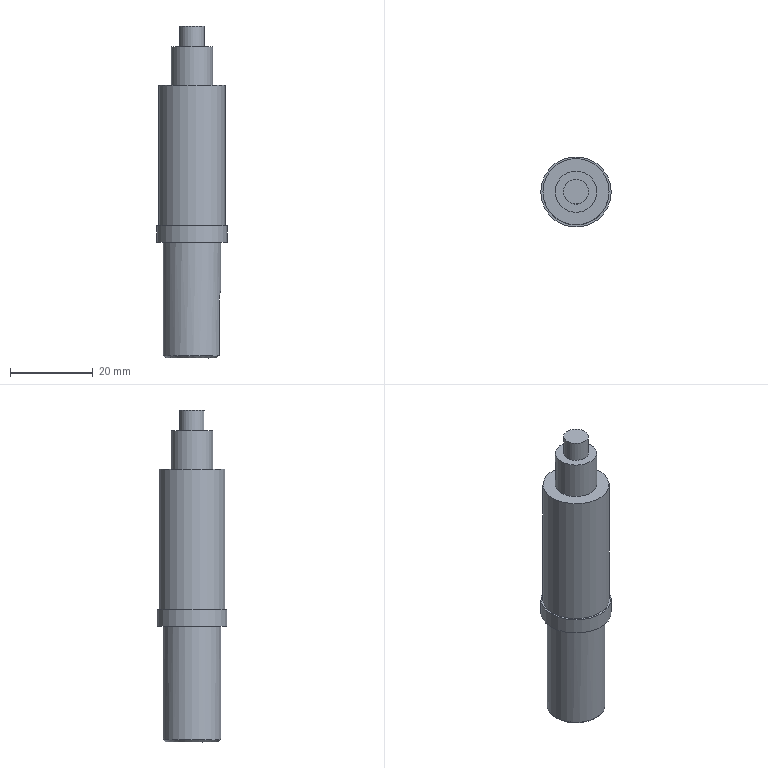Part | STEP file | 1 solid | 16 faces | box 17 x 17 x 80.2 mm | volume 12671 mm3 | plane 9 | cylinder 6 | cone 1 | commonest cylinder face diameters 5 x1 6 x1 10 x1 14 x1 16 x1 17 x1
STEP:
#1=CARTESIAN_POINT('',(0.,0.,0.));
#2=DIRECTION('',(0.,0.,1.));
#3=DIRECTION('',(1.,0.,0.));
#4=AXIS2_PLACEMENT_3D('',#1,#2,#3);
#5=CARTESIAN_POINT('',(8.,0.,-14.3));
#6=VERTEX_POINT('',#5);
#7=CARTESIAN_POINT('',(0.,0.,-14.3));
#8=DIRECTION('',(0.,0.,-1.));
#9=DIRECTION('',(1.,0.,0.));
#10=AXIS2_PLACEMENT_3D('',#7,#8,#9);
#11=CIRCLE('',#10,8.);
#12=CARTESIAN_POINT('',(0.,0.,-14.3));
#13=DIRECTION('',(0.,0.,1.));
#14=DIRECTION('',(1.,0.,0.));
#15=AXIS2_PLACEMENT_3D('',#12,#13,#14);
#16=CYLINDRICAL_SURFACE('',#15,8.);
#17=CARTESIAN_POINT('',(6.283,0.));
#18=DIRECTION('',(-1.,0.));
#19=VECTOR('',#18,1.);
#20=LINE('',#17,#19);
#21=(GEOMETRIC_REPRESENTATION_CONTEXT(2)PARAMETRIC_REPRESENTATION_CONTEXT()REPRESENTATION_CONTEXT('',''));
#22=DEFINITIONAL_REPRESENTATION('',(#20),#21);
#23=PCURVE('',#16,#22);
#24=CARTESIAN_POINT('',(0.,0.,-14.3));
#25=DIRECTION('',(0.,0.,1.));
#26=DIRECTION('',(1.,0.,0.));
#27=AXIS2_PLACEMENT_3D('',#24,#25,#26);
#28=PLANE('',#27);
#29=CARTESIAN_POINT('',(8.,0.));
#30=CARTESIAN_POINT('',(8.,-13.856));
#31=CARTESIAN_POINT('',(-4.,-6.928));
#32=CARTESIAN_POINT('',(-16.,0.));
#33=CARTESIAN_POINT('',(-4.,6.928));
#34=CARTESIAN_POINT('',(8.,13.856));
#35=CARTESIAN_POINT('',(8.,0.));
#36=(BOUNDED_CURVE()B_SPLINE_CURVE(2,(#29,#30,#31,#32,#33,#34,#35),.UNSPECIFIED.,.T.,.F.)B_SPLINE_CURVE_WITH_KNOTS((1,2,2,2,2,1),(-2.094,0.,2.094,4.189,6.283,8.378),.UNSPECIFIED.)CURVE()GEOMETRIC_REPRESENTATION_ITEM()RATIONAL_B_SPLINE_CURVE((1.,0.5,1.,0.5,1.,0.5,1.))REPRESENTATION_ITEM(''));
#37=(GEOMETRIC_REPRESENTATION_CONTEXT(2)PARAMETRIC_REPRESENTATION_CONTEXT()REPRESENTATION_CONTEXT('',''));
#38=DEFINITIONAL_REPRESENTATION('',(#36),#37);
#39=PCURVE('',#28,#38);
#40=SURFACE_CURVE('',#11,(#23,#39),.PCURVE_S1.);
#41=EDGE_CURVE('',#6,#6,#40,.T.);
#42=ORIENTED_EDGE('',*,*,#41,.T.);
#43=CARTESIAN_POINT('',(8.,0.,-48.3));
#44=VERTEX_POINT('',#43);
#45=CARTESIAN_POINT('',(8.,0.,-48.3));
#46=CARTESIAN_POINT('',(8.,0.,-14.3));
#47=B_SPLINE_CURVE_WITH_KNOTS('',1,(#45,#46),.UNSPECIFIED.,.F.,.F.,(2,2),(-34.,0.),.PIECEWISE_BEZIER_KNOTS.);
#48=CARTESIAN_POINT('',(0.,0.));
#49=DIRECTION('',(0.,1.));
#50=VECTOR('',#49,1.);
#51=LINE('',#48,#50);
#52=(GEOMETRIC_REPRESENTATION_CONTEXT(2)PARAMETRIC_REPRESENTATION_CONTEXT()REPRESENTATION_CONTEXT('',''));
#53=DEFINITIONAL_REPRESENTATION('',(#51),#52);
#54=PCURVE('',#16,#53);
#55=CARTESIAN_POINT('',(6.283,0.));
#56=DIRECTION('',(0.,1.));
#57=VECTOR('',#56,1.);
#58=LINE('',#55,#57);
#59=(GEOMETRIC_REPRESENTATION_CONTEXT(2)PARAMETRIC_REPRESENTATION_CONTEXT()REPRESENTATION_CONTEXT('',''));
#60=DEFINITIONAL_REPRESENTATION('',(#58),#59);
#61=PCURVE('',#16,#60);
#62=SEAM_CURVE('',#47,(#54,#61),.PCURVE_S1.);
#63=EDGE_CURVE('',#44,#6,#62,.T.);
#64=ORIENTED_EDGE('',*,*,#63,.F.);
#65=CARTESIAN_POINT('',(0.,0.,-48.3));
#66=DIRECTION('',(0.,0.,1.));
#67=DIRECTION('',(1.,0.,0.));
#68=AXIS2_PLACEMENT_3D('',#65,#66,#67);
#69=CIRCLE('',#68,8.);
#70=CARTESIAN_POINT('',(0.,-34.));
#71=DIRECTION('',(1.,0.));
#72=VECTOR('',#71,1.);
#73=LINE('',#70,#72);
#74=(GEOMETRIC_REPRESENTATION_CONTEXT(2)PARAMETRIC_REPRESENTATION_CONTEXT()REPRESENTATION_CONTEXT('',''));
#75=DEFINITIONAL_REPRESENTATION('',(#73),#74);
#76=PCURVE('',#16,#75);
#77=CARTESIAN_POINT('',(0.,0.,-48.3));
#78=DIRECTION('',(0.,0.,1.));
#79=DIRECTION('',(1.,0.,0.));
#80=AXIS2_PLACEMENT_3D('',#77,#78,#79);
#81=PLANE('',#80);
#82=CARTESIAN_POINT('',(0.,0.));
#83=DIRECTION('',(1.,0.));
#84=AXIS2_PLACEMENT_2D('',#82,#83);
#85=CIRCLE('',#84,8.);
#86=(GEOMETRIC_REPRESENTATION_CONTEXT(2)PARAMETRIC_REPRESENTATION_CONTEXT()REPRESENTATION_CONTEXT('',''));
#87=DEFINITIONAL_REPRESENTATION('',(#85),#86);
#88=PCURVE('',#81,#87);
#89=SURFACE_CURVE('',#69,(#76,#88),.PCURVE_S1.);
#90=EDGE_CURVE('',#44,#44,#89,.T.);
#91=ORIENTED_EDGE('',*,*,#90,.T.);
#92=ORIENTED_EDGE('',*,*,#63,.T.);
#93=EDGE_LOOP('',(#42,#64,#91,#92));
#94=FACE_BOUND('',#93,.T.);
#95=ADVANCED_FACE('',(#94),#16,.T.);
#96=CARTESIAN_POINT('',(5.,0.,-14.3));
#97=VERTEX_POINT('',#96);
#98=CARTESIAN_POINT('',(0.,0.,-14.3));
#99=DIRECTION('',(0.,0.,-1.));
#100=DIRECTION('',(1.,0.,0.));
#101=AXIS2_PLACEMENT_3D('',#98,#99,#100);
#102=CIRCLE('',#101,5.);
#103=CARTESIAN_POINT('',(5.,0.));
#104=CARTESIAN_POINT('',(5.,-8.66));
#105=CARTESIAN_POINT('',(-2.5,-4.33));
#106=CARTESIAN_POINT('',(-10.,0.));
#107=CARTESIAN_POINT('',(-2.5,4.33));
#108=CARTESIAN_POINT('',(5.,8.66));
#109=CARTESIAN_POINT('',(5.,0.));
#110=(BOUNDED_CURVE()B_SPLINE_CURVE(2,(#103,#104,#105,#106,#107,#108,#109),.UNSPECIFIED.,.T.,.F.)B_SPLINE_CURVE_WITH_KNOTS((1,2,2,2,2,1),(-2.094,0.,2.094,4.189,6.283,8.378),.UNSPECIFIED.)CURVE()GEOMETRIC_REPRESENTATION_ITEM()RATIONAL_B_SPLINE_CURVE((1.,0.5,1.,0.5,1.,0.5,1.))REPRESENTATION_ITEM(''));
#111=(GEOMETRIC_REPRESENTATION_CONTEXT(2)PARAMETRIC_REPRESENTATION_CONTEXT()REPRESENTATION_CONTEXT('',''));
#112=DEFINITIONAL_REPRESENTATION('',(#110),#111);
#113=PCURVE('',#28,#112);
#114=CARTESIAN_POINT('',(0.,0.,-5.));
#115=DIRECTION('',(0.,0.,1.));
#116=DIRECTION('',(1.,0.,0.));
#117=AXIS2_PLACEMENT_3D('',#114,#115,#116);
#118=CYLINDRICAL_SURFACE('',#117,5.);
#119=CARTESIAN_POINT('',(6.283,-9.3));
#120=DIRECTION('',(-1.,0.));
#121=VECTOR('',#120,1.);
#122=LINE('',#119,#121);
#123=(GEOMETRIC_REPRESENTATION_CONTEXT(2)PARAMETRIC_REPRESENTATION_CONTEXT()REPRESENTATION_CONTEXT('',''));
#124=DEFINITIONAL_REPRESENTATION('',(#122),#123);
#125=PCURVE('',#118,#124);
#126=SURFACE_CURVE('',#102,(#113,#125),.PCURVE_S1.);
#127=EDGE_CURVE('',#97,#97,#126,.T.);
#128=ORIENTED_EDGE('',*,*,#127,.T.);
#129=EDGE_LOOP('',(#128));
#130=FACE_BOUND('',#129,.T.);
#131=ORIENTED_EDGE('',*,*,#41,.F.);
#132=EDGE_LOOP('',(#131));
#133=FACE_BOUND('',#132,.T.);
#134=ADVANCED_FACE('',(#130,#133),#28,.T.);
#135=ORIENTED_EDGE('',*,*,#90,.F.);
#136=EDGE_LOOP('',(#135));
#137=FACE_BOUND('',#136,.T.);
#138=CARTESIAN_POINT('',(8.5,0.,-48.3));
#139=VERTEX_POINT('',#138);
#140=CARTESIAN_POINT('',(0.,0.,-48.3));
#141=DIRECTION('',(0.,0.,1.));
#142=DIRECTION('',(1.,0.,0.));
#143=AXIS2_PLACEMENT_3D('',#140,#141,#142);
#144=CIRCLE('',#143,8.5);
#145=CARTESIAN_POINT('',(0.,0.));
#146=DIRECTION('',(1.,0.));
#147=AXIS2_PLACEMENT_2D('',#145,#146);
#148=CIRCLE('',#147,8.5);
#149=(GEOMETRIC_REPRESENTATION_CONTEXT(2)PARAMETRIC_REPRESENTATION_CONTEXT()REPRESENTATION_CONTEXT('',''));
#150=DEFINITIONAL_REPRESENTATION('',(#148),#149);
#151=PCURVE('',#81,#150);
#152=CARTESIAN_POINT('',(0.,0.,0.));
#153=DIRECTION('',(0.,0.,1.));
#154=DIRECTION('',(1.,0.,0.));
#155=AXIS2_PLACEMENT_3D('',#152,#153,#154);
#156=CYLINDRICAL_SURFACE('',#155,8.5);
#157=CARTESIAN_POINT('',(0.,-48.3));
#158=DIRECTION('',(1.,0.));
#159=VECTOR('',#158,1.);
#160=LINE('',#157,#159);
#161=(GEOMETRIC_REPRESENTATION_CONTEXT(2)PARAMETRIC_REPRESENTATION_CONTEXT()REPRESENTATION_CONTEXT('',''));
#162=DEFINITIONAL_REPRESENTATION('',(#160),#161);
#163=PCURVE('',#156,#162);
#164=SURFACE_CURVE('',#144,(#151,#163),.PCURVE_S1.);
#165=EDGE_CURVE('',#139,#139,#164,.T.);
#166=ORIENTED_EDGE('',*,*,#165,.T.);
#167=EDGE_LOOP('',(#166));
#168=FACE_BOUND('',#167,.T.);
#169=ADVANCED_FACE('',(#137,#168),#81,.T.);
#170=CARTESIAN_POINT('',(5.,0.,-5.));
#171=VERTEX_POINT('',#170);
#172=CARTESIAN_POINT('',(0.,0.,-5.));
#173=DIRECTION('',(0.,0.,-1.));
#174=DIRECTION('',(1.,0.,0.));
#175=AXIS2_PLACEMENT_3D('',#172,#173,#174);
#176=CIRCLE('',#175,5.);
#177=CARTESIAN_POINT('',(6.283,0.));
#178=DIRECTION('',(-1.,0.));
#179=VECTOR('',#178,1.);
#180=LINE('',#177,#179);
#181=(GEOMETRIC_REPRESENTATION_CONTEXT(2)PARAMETRIC_REPRESENTATION_CONTEXT()REPRESENTATION_CONTEXT('',''));
#182=DEFINITIONAL_REPRESENTATION('',(#180),#181);
#183=PCURVE('',#118,#182);
#184=CARTESIAN_POINT('',(0.,0.,-5.));
#185=DIRECTION('',(0.,0.,1.));
#186=DIRECTION('',(1.,0.,0.));
#187=AXIS2_PLACEMENT_3D('',#184,#185,#186);
#188=PLANE('',#187);
#189=CARTESIAN_POINT('',(5.,0.));
#190=CARTESIAN_POINT('',(5.,-8.66));
#191=CARTESIAN_POINT('',(-2.5,-4.33));
#192=CARTESIAN_POINT('',(-10.,0.));
#193=CARTESIAN_POINT('',(-2.5,4.33));
#194=CARTESIAN_POINT('',(5.,8.66));
#195=CARTESIAN_POINT('',(5.,0.));
#196=(BOUNDED_CURVE()B_SPLINE_CURVE(2,(#189,#190,#191,#192,#193,#194,#195),.UNSPECIFIED.,.T.,.F.)B_SPLINE_CURVE_WITH_KNOTS((1,2,2,2,2,1),(-2.094,0.,2.094,4.189,6.283,8.378),.UNSPECIFIED.)CURVE()GEOMETRIC_REPRESENTATION_ITEM()RATIONAL_B_SPLINE_CURVE((1.,0.5,1.,0.5,1.,0.5,1.))REPRESENTATION_ITEM(''));
#197=(GEOMETRIC_REPRESENTATION_CONTEXT(2)PARAMETRIC_REPRESENTATION_CONTEXT()REPRESENTATION_CONTEXT('',''));
#198=DEFINITIONAL_REPRESENTATION('',(#196),#197);
#199=PCURVE('',#188,#198);
#200=SURFACE_CURVE('',#176,(#183,#199),.PCURVE_S1.);
#201=EDGE_CURVE('',#171,#171,#200,.T.);
#202=ORIENTED_EDGE('',*,*,#201,.T.);
#203=CARTESIAN_POINT('',(5.,0.,-14.3));
#204=CARTESIAN_POINT('',(5.,0.,-5.));
#205=B_SPLINE_CURVE_WITH_KNOTS('',1,(#203,#204),.UNSPECIFIED.,.F.,.F.,(2,2),(-9.3,0.),.PIECEWISE_BEZIER_KNOTS.);
#206=CARTESIAN_POINT('',(0.,0.));
#207=DIRECTION('',(0.,1.));
#208=VECTOR('',#207,1.);
#209=LINE('',#206,#208);
#210=(GEOMETRIC_REPRESENTATION_CONTEXT(2)PARAMETRIC_REPRESENTATION_CONTEXT()REPRESENTATION_CONTEXT('',''));
#211=DEFINITIONAL_REPRESENTATION('',(#209),#210);
#212=PCURVE('',#118,#211);
#213=CARTESIAN_POINT('',(6.283,0.));
#214=DIRECTION('',(0.,1.));
#215=VECTOR('',#214,1.);
#216=LINE('',#213,#215);
#217=(GEOMETRIC_REPRESENTATION_CONTEXT(2)PARAMETRIC_REPRESENTATION_CONTEXT()REPRESENTATION_CONTEXT('',''));
#218=DEFINITIONAL_REPRESENTATION('',(#216),#217);
#219=PCURVE('',#118,#218);
#220=SEAM_CURVE('',#205,(#212,#219),.PCURVE_S1.);
#221=EDGE_CURVE('',#97,#171,#220,.T.);
#222=ORIENTED_EDGE('',*,*,#221,.F.);
#223=ORIENTED_EDGE('',*,*,#127,.F.);
#224=ORIENTED_EDGE('',*,*,#221,.T.);
#225=EDGE_LOOP('',(#202,#222,#223,#224));
#226=FACE_BOUND('',#225,.T.);
#227=ADVANCED_FACE('',(#226),#118,.T.);
#228=CARTESIAN_POINT('',(8.5,0.,-52.2));
#229=VERTEX_POINT('',#228);
#230=CARTESIAN_POINT('',(0.,0.,-52.2));
#231=DIRECTION('',(0.,0.,1.));
#232=DIRECTION('',(1.,0.,0.));
#233=AXIS2_PLACEMENT_3D('',#230,#231,#232);
#234=CIRCLE('',#233,8.5);
#235=CARTESIAN_POINT('',(0.,-52.2));
#236=DIRECTION('',(1.,0.));
#237=VECTOR('',#236,1.);
#238=LINE('',#235,#237);
#239=(GEOMETRIC_REPRESENTATION_CONTEXT(2)PARAMETRIC_REPRESENTATION_CONTEXT()REPRESENTATION_CONTEXT('',''));
#240=DEFINITIONAL_REPRESENTATION('',(#238),#239);
#241=PCURVE('',#156,#240);
#242=CARTESIAN_POINT('',(0.,0.,-52.2));
#243=DIRECTION('',(0.,0.,-1.));
#244=DIRECTION('',(-1.,0.,0.));
#245=AXIS2_PLACEMENT_3D('',#242,#243,#244);
#246=PLANE('',#245);
#247=CARTESIAN_POINT('',(-8.5,0.));
#248=CARTESIAN_POINT('',(-8.5,14.722));
#249=CARTESIAN_POINT('',(4.25,7.361));
#250=CARTESIAN_POINT('',(17.,0.));
#251=CARTESIAN_POINT('',(4.25,-7.361));
#252=CARTESIAN_POINT('',(-8.5,-14.722));
#253=CARTESIAN_POINT('',(-8.5,0.));
#254=(BOUNDED_CURVE()B_SPLINE_CURVE(2,(#247,#248,#249,#250,#251,#252,#253),.UNSPECIFIED.,.T.,.F.)B_SPLINE_CURVE_WITH_KNOTS((1,2,2,2,2,1),(-2.094,0.,2.094,4.189,6.283,8.378),.UNSPECIFIED.)CURVE()GEOMETRIC_REPRESENTATION_ITEM()RATIONAL_B_SPLINE_CURVE((1.,0.5,1.,0.5,1.,0.5,1.))REPRESENTATION_ITEM(''));
#255=(GEOMETRIC_REPRESENTATION_CONTEXT(2)PARAMETRIC_REPRESENTATION_CONTEXT()REPRESENTATION_CONTEXT('',''));
#256=DEFINITIONAL_REPRESENTATION('',(#254),#255);
#257=PCURVE('',#246,#256);
#258=SURFACE_CURVE('',#234,(#241,#257),.PCURVE_S1.);
#259=EDGE_CURVE('',#229,#229,#258,.T.);
#260=ORIENTED_EDGE('',*,*,#259,.T.);
#261=CARTESIAN_POINT('',(8.5,0.,-52.2));
#262=CARTESIAN_POINT('',(8.5,0.,-48.3));
#263=B_SPLINE_CURVE_WITH_KNOTS('',1,(#261,#262),.UNSPECIFIED.,.F.,.F.,(2,2),(-52.2,-48.3),.PIECEWISE_BEZIER_KNOTS.);
#264=CARTESIAN_POINT('',(6.283,0.));
#265=DIRECTION('',(0.,1.));
#266=VECTOR('',#265,1.);
#267=LINE('',#264,#266);
#268=(GEOMETRIC_REPRESENTATION_CONTEXT(2)PARAMETRIC_REPRESENTATION_CONTEXT()REPRESENTATION_CONTEXT('',''));
#269=DEFINITIONAL_REPRESENTATION('',(#267),#268);
#270=PCURVE('',#156,#269);
#271=CARTESIAN_POINT('',(0.,0.));
#272=DIRECTION('',(0.,1.));
#273=VECTOR('',#272,1.);
#274=LINE('',#271,#273);
#275=(GEOMETRIC_REPRESENTATION_CONTEXT(2)PARAMETRIC_REPRESENTATION_CONTEXT()REPRESENTATION_CONTEXT('',''));
#276=DEFINITIONAL_REPRESENTATION('',(#274),#275);
#277=PCURVE('',#156,#276);
#278=SEAM_CURVE('',#263,(#270,#277),.PCURVE_S1.);
#279=EDGE_CURVE('',#229,#139,#278,.T.);
#280=ORIENTED_EDGE('',*,*,#279,.T.);
#281=ORIENTED_EDGE('',*,*,#165,.F.);
#282=ORIENTED_EDGE('',*,*,#279,.F.);
#283=EDGE_LOOP('',(#260,#280,#281,#282));
#284=FACE_BOUND('',#283,.T.);
#285=ADVANCED_FACE('',(#284),#156,.T.);
#286=CARTESIAN_POINT('',(3.,0.,-5.));
#287=VERTEX_POINT('',#286);
#288=CARTESIAN_POINT('',(0.,0.,-5.));
#289=DIRECTION('',(0.,0.,-1.));
#290=DIRECTION('',(1.,0.,0.));
#291=AXIS2_PLACEMENT_3D('',#288,#289,#290);
#292=CIRCLE('',#291,3.);
#293=CARTESIAN_POINT('',(3.,0.));
#294=CARTESIAN_POINT('',(3.,-5.196));
#295=CARTESIAN_POINT('',(-1.5,-2.598));
#296=CARTESIAN_POINT('',(-6.,0.));
#297=CARTESIAN_POINT('',(-1.5,2.598));
#298=CARTESIAN_POINT('',(3.,5.196));
#299=CARTESIAN_POINT('',(3.,0.));
#300=(BOUNDED_CURVE()B_SPLINE_CURVE(2,(#293,#294,#295,#296,#297,#298,#299),.UNSPECIFIED.,.T.,.F.)B_SPLINE_CURVE_WITH_KNOTS((1,2,2,2,2,1),(-2.094,0.,2.094,4.189,6.283,8.378),.UNSPECIFIED.)CURVE()GEOMETRIC_REPRESENTATION_ITEM()RATIONAL_B_SPLINE_CURVE((1.,0.5,1.,0.5,1.,0.5,1.))REPRESENTATION_ITEM(''));
#301=(GEOMETRIC_REPRESENTATION_CONTEXT(2)PARAMETRIC_REPRESENTATION_CONTEXT()REPRESENTATION_CONTEXT('',''));
#302=DEFINITIONAL_REPRESENTATION('',(#300),#301);
#303=PCURVE('',#188,#302);
#304=CARTESIAN_POINT('',(0.,0.,0.));
#305=DIRECTION('',(0.,0.,1.));
#306=DIRECTION('',(1.,0.,0.));
#307=AXIS2_PLACEMENT_3D('',#304,#305,#306);
#308=CYLINDRICAL_SURFACE('',#307,3.);
#309=CARTESIAN_POINT('',(6.283,-5.));
#310=DIRECTION('',(-1.,0.));
#311=VECTOR('',#310,1.);
#312=LINE('',#309,#311);
#313=(GEOMETRIC_REPRESENTATION_CONTEXT(2)PARAMETRIC_REPRESENTATION_CONTEXT()REPRESENTATION_CONTEXT('',''));
#314=DEFINITIONAL_REPRESENTATION('',(#312),#313);
#315=PCURVE('',#308,#314);
#316=SURFACE_CURVE('',#292,(#303,#315),.PCURVE_S1.);
#317=EDGE_CURVE('',#287,#287,#316,.T.);
#318=ORIENTED_EDGE('',*,*,#317,.T.);
#319=EDGE_LOOP('',(#318));
#320=FACE_BOUND('',#319,.T.);
#321=ORIENTED_EDGE('',*,*,#201,.F.);
#322=EDGE_LOOP('',(#321));
#323=FACE_BOUND('',#322,.T.);
#324=ADVANCED_FACE('',(#320,#323),#188,.T.);
#325=CARTESIAN_POINT('',(-7.,0.,-52.2));
#326=VERTEX_POINT('',#325);
#327=CARTESIAN_POINT('',(0.,0.,-52.2));
#328=DIRECTION('',(0.,0.,1.));
#329=DIRECTION('',(-1.,0.,0.));
#330=AXIS2_PLACEMENT_3D('',#327,#328,#329);
#331=CIRCLE('',#330,7.);
#332=CARTESIAN_POINT('',(7.,0.));
#333=CARTESIAN_POINT('',(7.,-12.124));
#334=CARTESIAN_POINT('',(-3.5,-6.062));
#335=CARTESIAN_POINT('',(-14.,0.));
#336=CARTESIAN_POINT('',(-3.5,6.062));
#337=CARTESIAN_POINT('',(7.,12.124));
#338=CARTESIAN_POINT('',(7.,0.));
#339=(BOUNDED_CURVE()B_SPLINE_CURVE(2,(#332,#333,#334,#335,#336,#337,#338),.UNSPECIFIED.,.T.,.F.)B_SPLINE_CURVE_WITH_KNOTS((1,2,2,2,2,1),(-2.094,0.,2.094,4.189,6.283,8.378),.UNSPECIFIED.)CURVE()GEOMETRIC_REPRESENTATION_ITEM()RATIONAL_B_SPLINE_CURVE((1.,0.5,1.,0.5,1.,0.5,1.))REPRESENTATION_ITEM(''));
#340=(GEOMETRIC_REPRESENTATION_CONTEXT(2)PARAMETRIC_REPRESENTATION_CONTEXT()REPRESENTATION_CONTEXT('',''));
#341=DEFINITIONAL_REPRESENTATION('',(#339),#340);
#342=PCURVE('',#246,#341);
#343=CARTESIAN_POINT('',(0.,0.,-80.2));
#344=DIRECTION('',(0.,0.,-1.));
#345=DIRECTION('',(-1.,0.,0.));
#346=AXIS2_PLACEMENT_3D('',#343,#344,#345);
#347=CYLINDRICAL_SURFACE('',#346,7.);
#348=CARTESIAN_POINT('',(6.283,-28.));
#349=DIRECTION('',(-1.,0.));
#350=VECTOR('',#349,1.);
#351=LINE('',#348,#350);
#352=(GEOMETRIC_REPRESENTATION_CONTEXT(2)PARAMETRIC_REPRESENTATION_CONTEXT()REPRESENTATION_CONTEXT('',''));
#353=DEFINITIONAL_REPRESENTATION('',(#351),#352);
#354=PCURVE('',#347,#353);
#355=SURFACE_CURVE('',#331,(#342,#354),.PCURVE_S1.);
#356=EDGE_CURVE('',#326,#326,#355,.T.);
#357=ORIENTED_EDGE('',*,*,#356,.T.);
#358=EDGE_LOOP('',(#357));
#359=FACE_BOUND('',#358,.T.);
#360=ORIENTED_EDGE('',*,*,#259,.F.);
#361=EDGE_LOOP('',(#360));
#362=FACE_BOUND('',#361,.T.);
#363=ADVANCED_FACE('',(#359,#362),#246,.T.);
#364=CARTESIAN_POINT('',(3.,0.,0.));
#365=VERTEX_POINT('',#364);
#366=CARTESIAN_POINT('',(0.,0.,0.));
#367=DIRECTION('',(0.,0.,-1.));
#368=DIRECTION('',(1.,0.,0.));
#369=AXIS2_PLACEMENT_3D('',#366,#367,#368);
#370=CIRCLE('',#369,3.);
#371=CARTESIAN_POINT('',(6.283,0.));
#372=DIRECTION('',(-1.,0.));
#373=VECTOR('',#372,1.);
#374=LINE('',#371,#373);
#375=(GEOMETRIC_REPRESENTATION_CONTEXT(2)PARAMETRIC_REPRESENTATION_CONTEXT()REPRESENTATION_CONTEXT('',''));
#376=DEFINITIONAL_REPRESENTATION('',(#374),#375);
#377=PCURVE('',#308,#376);
#378=CARTESIAN_POINT('',(0.,0.,0.));
#379=DIRECTION('',(0.,0.,1.));
#380=DIRECTION('',(1.,0.,0.));
#381=AXIS2_PLACEMENT_3D('',#378,#379,#380);
#382=PLANE('',#381);
#383=CARTESIAN_POINT('',(3.,0.));
#384=CARTESIAN_POINT('',(3.,-5.196));
#385=CARTESIAN_POINT('',(-1.5,-2.598));
#386=CARTESIAN_POINT('',(-6.,0.));
#387=CARTESIAN_POINT('',(-1.5,2.598));
#388=CARTESIAN_POINT('',(3.,5.196));
#389=CARTESIAN_POINT('',(3.,0.));
#390=(BOUNDED_CURVE()B_SPLINE_CURVE(2,(#383,#384,#385,#386,#387,#388,#389),.UNSPECIFIED.,.T.,.F.)B_SPLINE_CURVE_WITH_KNOTS((1,2,2,2,2,1),(-2.094,0.,2.094,4.189,6.283,8.378),.UNSPECIFIED.)CURVE()GEOMETRIC_REPRESENTATION_ITEM()RATIONAL_B_SPLINE_CURVE((1.,0.5,1.,0.5,1.,0.5,1.))REPRESENTATION_ITEM(''));
#391=(GEOMETRIC_REPRESENTATION_CONTEXT(2)PARAMETRIC_REPRESENTATION_CONTEXT()REPRESENTATION_CONTEXT('',''));
#392=DEFINITIONAL_REPRESENTATION('',(#390),#391);
#393=PCURVE('',#382,#392);
#394=SURFACE_CURVE('',#370,(#377,#393),.PCURVE_S1.);
#395=EDGE_CURVE('',#365,#365,#394,.T.);
#396=ORIENTED_EDGE('',*,*,#395,.T.);
#397=CARTESIAN_POINT('',(3.,0.,-5.));
#398=CARTESIAN_POINT('',(3.,0.,0.));
#399=B_SPLINE_CURVE_WITH_KNOTS('',1,(#397,#398),.UNSPECIFIED.,.F.,.F.,(2,2),(-5.,0.),.PIECEWISE_BEZIER_KNOTS.);
#400=CARTESIAN_POINT('',(0.,0.));
#401=DIRECTION('',(0.,1.));
#402=VECTOR('',#401,1.);
#403=LINE('',#400,#402);
#404=(GEOMETRIC_REPRESENTATION_CONTEXT(2)PARAMETRIC_REPRESENTATION_CONTEXT()REPRESENTATION_CONTEXT('',''));
#405=DEFINITIONAL_REPRESENTATION('',(#403),#404);
#406=PCURVE('',#308,#405);
#407=CARTESIAN_POINT('',(6.283,0.));
#408=DIRECTION('',(0.,1.));
#409=VECTOR('',#408,1.);
#410=LINE('',#407,#409);
#411=(GEOMETRIC_REPRESENTATION_CONTEXT(2)PARAMETRIC_REPRESENTATION_CONTEXT()REPRESENTATION_CONTEXT('',''));
#412=DEFINITIONAL_REPRESENTATION('',(#410),#411);
#413=PCURVE('',#308,#412);
#414=SEAM_CURVE('',#399,(#406,#413),.PCURVE_S1.);
#415=EDGE_CURVE('',#287,#365,#414,.T.);
#416=ORIENTED_EDGE('',*,*,#415,.F.);
#417=ORIENTED_EDGE('',*,*,#317,.F.);
#418=ORIENTED_EDGE('',*,*,#415,.T.);
#419=EDGE_LOOP('',(#396,#416,#417,#418));
#420=FACE_BOUND('',#419,.T.);
#421=ADVANCED_FACE('',(#420),#308,.T.);
#422=CARTESIAN_POINT('',(6.538,-2.5,-79.7));
#423=VERTEX_POINT('',#422);
#424=CARTESIAN_POINT('',(6.538,-2.5,-66.2));
#425=VERTEX_POINT('',#424);
#426=CARTESIAN_POINT('',(6.538,-2.5,-80.2));
#427=DIRECTION('',(0.,0.,1.));
#428=VECTOR('',#427,1.);
#429=LINE('',#426,#428);
#430=CARTESIAN_POINT('',(3.507,0.));
#431=DIRECTION('',(0.,-1.));
#432=VECTOR('',#431,1.);
#433=LINE('',#430,#432);
#434=(GEOMETRIC_REPRESENTATION_CONTEXT(2)PARAMETRIC_REPRESENTATION_CONTEXT()REPRESENTATION_CONTEXT('',''));
#435=DEFINITIONAL_REPRESENTATION('',(#433),#434);
#436=PCURVE('',#347,#435);
#437=CARTESIAN_POINT('',(7.,-2.5,-66.2));
#438=DIRECTION('',(0.,-1.,0.));
#439=DIRECTION('',(0.,0.,-1.));
#440=AXIS2_PLACEMENT_3D('',#437,#438,#439);
#441=PLANE('',#440);
#442=CARTESIAN_POINT('',(14.,-0.4617));
#443=DIRECTION('',(-1.,0.));
#444=VECTOR('',#443,1.);
#445=LINE('',#442,#444);
#446=(GEOMETRIC_REPRESENTATION_CONTEXT(2)PARAMETRIC_REPRESENTATION_CONTEXT()REPRESENTATION_CONTEXT('',''));
#447=DEFINITIONAL_REPRESENTATION('',(#445),#446);
#448=PCURVE('',#441,#447);
#449=SURFACE_CURVE('',#429,(#436,#448),.PCURVE_S1.);
#450=EDGE_CURVE('',#423,#425,#449,.T.);
#451=ORIENTED_EDGE('',*,*,#450,.T.);
#452=CARTESIAN_POINT('',(6.538,2.5,-66.2));
#453=VERTEX_POINT('',#452);
#454=CARTESIAN_POINT('',(6.538,-2.5,-66.2));
#455=CARTESIAN_POINT('',(6.538,-2.5,-66.033));
#456=CARTESIAN_POINT('',(6.545,-2.484,-65.87));
#457=CARTESIAN_POINT('',(6.569,-2.419,-65.549));
#458=CARTESIAN_POINT('',(6.587,-2.371,-65.389));
#459=CARTESIAN_POINT('',(6.631,-2.245,-65.088));
#460=CARTESIAN_POINT('',(6.656,-2.168,-64.945));
#461=CARTESIAN_POINT('',(6.713,-1.987,-64.674));
#462=CARTESIAN_POINT('',(6.743,-1.883,-64.547));
#463=CARTESIAN_POINT('',(6.833,-1.54,-64.204));
#464=CARTESIAN_POINT('',(6.892,-1.264,-64.019));
#465=CARTESIAN_POINT('',(6.954,-0.8135,-63.83));
#466=CARTESIAN_POINT('',(6.971,-0.6548,-63.782));
#467=CARTESIAN_POINT('',(6.994,-0.3308,-63.716));
#468=CARTESIAN_POINT('',(7.,-0.1666,-63.7));
#469=CARTESIAN_POINT('',(7.,0.1665,-63.7));
#470=CARTESIAN_POINT('',(6.994,0.3301,-63.716));
#471=CARTESIAN_POINT('',(6.971,0.6513,-63.781));
#472=CARTESIAN_POINT('',(6.955,0.8108,-63.829));
#473=CARTESIAN_POINT('',(6.913,1.113,-63.955));
#474=CARTESIAN_POINT('',(6.888,1.256,-64.032));
#475=CARTESIAN_POINT('',(6.833,1.527,-64.214));
#476=CARTESIAN_POINT('',(6.803,1.654,-64.318));
#477=CARTESIAN_POINT('',(6.713,1.996,-64.661));
#478=CARTESIAN_POINT('',(6.653,2.182,-64.937));
#479=CARTESIAN_POINT('',(6.587,2.37,-65.387));
#480=CARTESIAN_POINT('',(6.569,2.418,-65.545));
#481=CARTESIAN_POINT('',(6.545,2.484,-65.869));
#482=CARTESIAN_POINT('',(6.538,2.5,-66.033));
#483=CARTESIAN_POINT('',(6.538,2.5,-66.2));
#484=B_SPLINE_CURVE_WITH_KNOTS('',3,(#454,#455,#456,#457,#458,#459,#460,#461,#462,#463,#464,#465,#466,#467,#468,#469,#470,#471,#472,#473,#474,#475,#476,#477,#478,#479,#480,#481,#482,#483),.UNSPECIFIED.,.F.,.F.,(4,2,2,2,2,2,2,2,2,2,2,2,2,2,4),(-0.003938,-0.003446,-0.002954,-0.002462,-0.001969,-0.0009846,-0.0004923,-0.000000015,0.0004923,0.0009846,0.001477,0.001969,0.002954,0.003446,0.003938),.UNSPECIFIED.);
#485=CARTESIAN_POINT('',(3.507,-14.));
#486=CARTESIAN_POINT('',(3.507,-14.04));
#487=CARTESIAN_POINT('',(3.507,-14.121));
#488=CARTESIAN_POINT('',(3.505,-14.24));
#489=CARTESIAN_POINT('',(3.503,-14.359));
#490=CARTESIAN_POINT('',(3.5,-14.476));
#491=CARTESIAN_POINT('',(3.496,-14.593));
#492=CARTESIAN_POINT('',(3.491,-14.708));
#493=CARTESIAN_POINT('',(3.486,-14.823));
#494=CARTESIAN_POINT('',(3.479,-14.934));
#495=CARTESIAN_POINT('',(3.472,-15.044));
#496=CARTESIAN_POINT('',(3.464,-15.15));
#497=CARTESIAN_POINT('',(3.456,-15.253));
#498=CARTESIAN_POINT('',(3.447,-15.354));
#499=CARTESIAN_POINT('',(3.437,-15.452));
#500=CARTESIAN_POINT('',(3.426,-15.547));
#501=CARTESIAN_POINT('',(3.415,-15.638));
#502=CARTESIAN_POINT('',(3.403,-15.726));
#503=CARTESIAN_POINT('',(3.391,-15.809));
#504=CARTESIAN_POINT('',(3.378,-15.888));
#505=CARTESIAN_POINT('',(3.365,-15.963));
#506=CARTESIAN_POINT('',(3.351,-16.034));
#507=CARTESIAN_POINT('',(3.337,-16.101));
#508=CARTESIAN_POINT('',(3.322,-16.163));
#509=CARTESIAN_POINT('',(3.307,-16.22));
#510=CARTESIAN_POINT('',(3.291,-16.272));
#511=CARTESIAN_POINT('',(3.276,-16.319));
#512=CARTESIAN_POINT('',(3.26,-16.361));
#513=CARTESIAN_POINT('',(3.243,-16.398));
#514=CARTESIAN_POINT('',(3.227,-16.429));
#515=CARTESIAN_POINT('',(3.21,-16.455));
#516=CARTESIAN_POINT('',(3.193,-16.475));
#517=CARTESIAN_POINT('',(3.176,-16.489));
#518=CARTESIAN_POINT('',(3.159,-16.498));
#519=CARTESIAN_POINT('',(3.142,-16.501));
#520=CARTESIAN_POINT('',(3.124,-16.498));
#521=CARTESIAN_POINT('',(3.107,-16.489));
#522=CARTESIAN_POINT('',(3.09,-16.475));
#523=CARTESIAN_POINT('',(3.074,-16.455));
#524=CARTESIAN_POINT('',(3.057,-16.43));
#525=CARTESIAN_POINT('',(3.04,-16.398));
#526=CARTESIAN_POINT('',(3.024,-16.362));
#527=CARTESIAN_POINT('',(3.008,-16.32));
#528=CARTESIAN_POINT('',(2.992,-16.273));
#529=CARTESIAN_POINT('',(2.977,-16.221));
#530=CARTESIAN_POINT('',(2.962,-16.164));
#531=CARTESIAN_POINT('',(2.947,-16.102));
#532=CARTESIAN_POINT('',(2.933,-16.036));
#533=CARTESIAN_POINT('',(2.919,-15.965));
#534=CARTESIAN_POINT('',(2.905,-15.889));
#535=CARTESIAN_POINT('',(2.892,-15.809));
#536=CARTESIAN_POINT('',(2.88,-15.726));
#537=CARTESIAN_POINT('',(2.868,-15.639));
#538=CARTESIAN_POINT('',(2.857,-15.548));
#539=CARTESIAN_POINT('',(2.847,-15.454));
#540=CARTESIAN_POINT('',(2.837,-15.356));
#541=CARTESIAN_POINT('',(2.827,-15.255));
#542=CARTESIAN_POINT('',(2.819,-15.151));
#543=CARTESIAN_POINT('',(2.811,-15.045));
#544=CARTESIAN_POINT('',(2.804,-14.936));
#545=CARTESIAN_POINT('',(2.798,-14.825));
#546=CARTESIAN_POINT('',(2.792,-14.711));
#547=CARTESIAN_POINT('',(2.787,-14.596));
#548=CARTESIAN_POINT('',(2.783,-14.478));
#549=CARTESIAN_POINT('',(2.78,-14.36));
#550=CARTESIAN_POINT('',(2.778,-14.241));
#551=CARTESIAN_POINT('',(2.777,-14.121));
#552=CARTESIAN_POINT('',(2.776,-14.04));
#553=CARTESIAN_POINT('',(2.776,-14.));
#554=B_SPLINE_CURVE_WITH_KNOTS('',3,(#485,#486,#487,#488,#489,#490,#491,#492,#493,#494,#495,#496,#497,#498,#499,#500,#501,#502,#503,#504,#505,#506,#507,#508,#509,#510,#511,#512,#513,#514,#515,#516,#517,#518,#519,#520,#521,#522,#523,#524,#525,#526,#527,#528,#529,#530,#531,#532,#533,#534,#535,#536,#537,#538,#539,#540,#541,#542,#543,#544,#545,#546,#547,#548,#549,#550,#551,#552,#553),.UNSPECIFIED.,.F.,.F.,(4,1,1,1,1,1,1,1,1,1,1,1,1,1,1,1,1,1,1,1,1,1,1,1,1,1,1,1,1,1,1,1,1,1,1,1,1,1,1,1,1,1,1,1,1,1,1,1,1,1,1,1,1,1,1,1,1,1,1,1,1,1,1,1,1,1,4),(-0.003938,-0.003819,-0.0037,-0.00358,-0.003461,-0.003342,-0.003222,-0.003103,-0.002984,-0.002864,-0.002745,-0.002626,-0.002506,-0.002387,-0.002268,-0.002148,-0.002029,-0.00191,-0.00179,-0.001671,-0.001552,-0.001432,-0.001313,-0.001193,-0.001074,-0.0009548,-0.0008354,-0.0007161,-0.0005967,-0.0004774,-0.0003581,-0.0002387,-0.0001194,-0.000000015,0.0001193,0.0002387,0.000358,0.0004774,0.0005967,0.0007161,0.0008354,0.0009548,0.001074,0.001193,0.001313,0.001432,0.001551,0.001671,0.00179,0.00191,0.002029,0.002148,0.002268,0.002387,0.002506,0.002626,0.002745,0.002864,0.002984,0.003103,0.003222,0.003342,0.003461,0.00358,0.0037,0.003819,0.003938),.UNSPECIFIED.);
#555=(GEOMETRIC_REPRESENTATION_CONTEXT(2)PARAMETRIC_REPRESENTATION_CONTEXT()REPRESENTATION_CONTEXT('',''));
#556=DEFINITIONAL_REPRESENTATION('',(#554),#555);
#557=PCURVE('',#347,#556);
#558=CARTESIAN_POINT('',(7.,0.,-66.2));
#559=DIRECTION('',(1.,0.,0.));
#560=DIRECTION('',(0.,0.,-1.));
#561=AXIS2_PLACEMENT_3D('',#558,#559,#560);
#562=CYLINDRICAL_SURFACE('',#561,2.5);
#563=CARTESIAN_POINT('',(4.712,-0.4617));
#564=CARTESIAN_POINT('',(4.696,-0.4617));
#565=CARTESIAN_POINT('',(4.664,-0.4609));
#566=CARTESIAN_POINT('',(4.616,-0.4576));
#567=CARTESIAN_POINT('',(4.568,-0.4522));
#568=CARTESIAN_POINT('',(4.521,-0.4447));
#569=CARTESIAN_POINT('',(4.473,-0.4352));
#570=CARTESIAN_POINT('',(4.425,-0.4237));
#571=CARTESIAN_POINT('',(4.377,-0.4104));
#572=CARTESIAN_POINT('',(4.329,-0.3955));
#573=CARTESIAN_POINT('',(4.282,-0.3792));
#574=CARTESIAN_POINT('',(4.235,-0.3616));
#575=CARTESIAN_POINT('',(4.187,-0.3429));
#576=CARTESIAN_POINT('',(4.14,-0.3232));
#577=CARTESIAN_POINT('',(4.093,-0.3026));
#578=CARTESIAN_POINT('',(4.045,-0.2813));
#579=CARTESIAN_POINT('',(3.998,-0.2597));
#580=CARTESIAN_POINT('',(3.951,-0.2379));
#581=CARTESIAN_POINT('',(3.904,-0.2162));
#582=CARTESIAN_POINT('',(3.857,-0.1946));
#583=CARTESIAN_POINT('',(3.81,-0.1734));
#584=CARTESIAN_POINT('',(3.762,-0.1526));
#585=CARTESIAN_POINT('',(3.715,-0.1326));
#586=CARTESIAN_POINT('',(3.667,-0.1133));
#587=CARTESIAN_POINT('',(3.62,-0.09516));
#588=CARTESIAN_POINT('',(3.573,-0.07819));
#589=CARTESIAN_POINT('',(3.525,-0.06265));
#590=CARTESIAN_POINT('',(3.478,-0.04853));
#591=CARTESIAN_POINT('',(3.43,-0.03596));
#592=CARTESIAN_POINT('',(3.382,-0.02507));
#593=CARTESIAN_POINT('',(3.334,-0.01602));
#594=CARTESIAN_POINT('',(3.286,-0.008921));
#595=CARTESIAN_POINT('',(3.238,-0.0038));
#596=CARTESIAN_POINT('',(3.19,-0.0006979));
#597=CARTESIAN_POINT('',(3.142,0.0003488));
#598=CARTESIAN_POINT('',(3.093,-0.0006972));
#599=CARTESIAN_POINT('',(3.045,-0.003785));
#600=CARTESIAN_POINT('',(2.998,-0.008869));
#601=CARTESIAN_POINT('',(2.95,-0.01589));
#602=CARTESIAN_POINT('',(2.902,-0.02484));
#603=CARTESIAN_POINT('',(2.854,-0.03567));
#604=CARTESIAN_POINT('',(2.806,-0.04824));
#605=CARTESIAN_POINT('',(2.759,-0.06239));
#606=CARTESIAN_POINT('',(2.711,-0.07799));
#607=CARTESIAN_POINT('',(2.664,-0.09487));
#608=CARTESIAN_POINT('',(2.616,-0.1129));
#609=CARTESIAN_POINT('',(2.569,-0.1321));
#610=CARTESIAN_POINT('',(2.522,-0.1522));
#611=CARTESIAN_POINT('',(2.474,-0.173));
#612=CARTESIAN_POINT('',(2.427,-0.1944));
#613=CARTESIAN_POINT('',(2.38,-0.216));
#614=CARTESIAN_POINT('',(2.333,-0.2377));
#615=CARTESIAN_POINT('',(2.286,-0.2595));
#616=CARTESIAN_POINT('',(2.238,-0.281));
#617=CARTESIAN_POINT('',(2.191,-0.3021));
#618=CARTESIAN_POINT('',(2.144,-0.3227));
#619=CARTESIAN_POINT('',(2.096,-0.3425));
#620=CARTESIAN_POINT('',(2.049,-0.3613));
#621=CARTESIAN_POINT('',(2.002,-0.379));
#622=CARTESIAN_POINT('',(1.955,-0.3953));
#623=CARTESIAN_POINT('',(1.907,-0.4101));
#624=CARTESIAN_POINT('',(1.859,-0.4234));
#625=CARTESIAN_POINT('',(1.811,-0.4349));
#626=CARTESIAN_POINT('',(1.763,-0.4445));
#627=CARTESIAN_POINT('',(1.715,-0.4521));
#628=CARTESIAN_POINT('',(1.667,-0.4576));
#629=CARTESIAN_POINT('',(1.619,-0.4609));
#630=CARTESIAN_POINT('',(1.587,-0.4617));
#631=CARTESIAN_POINT('',(1.571,-0.4617));
#632=B_SPLINE_CURVE_WITH_KNOTS('',3,(#563,#564,#565,#566,#567,#568,#569,#570,#571,#572,#573,#574,#575,#576,#577,#578,#579,#580,#581,#582,#583,#584,#585,#586,#587,#588,#589,#590,#591,#592,#593,#594,#595,#596,#597,#598,#599,#600,#601,#602,#603,#604,#605,#606,#607,#608,#609,#610,#611,#612,#613,#614,#615,#616,#617,#618,#619,#620,#621,#622,#623,#624,#625,#626,#627,#628,#629,#630,#631),.UNSPECIFIED.,.F.,.F.,(4,1,1,1,1,1,1,1,1,1,1,1,1,1,1,1,1,1,1,1,1,1,1,1,1,1,1,1,1,1,1,1,1,1,1,1,1,1,1,1,1,1,1,1,1,1,1,1,1,1,1,1,1,1,1,1,1,1,1,1,1,1,1,1,1,1,4),(-0.003938,-0.003819,-0.0037,-0.00358,-0.003461,-0.003342,-0.003222,-0.003103,-0.002984,-0.002864,-0.002745,-0.002626,-0.002506,-0.002387,-0.002268,-0.002148,-0.002029,-0.00191,-0.00179,-0.001671,-0.001552,-0.001432,-0.001313,-0.001193,-0.001074,-0.0009548,-0.0008354,-0.0007161,-0.0005967,-0.0004774,-0.0003581,-0.0002387,-0.0001194,-0.000000015,0.0001193,0.0002387,0.000358,0.0004774,0.0005967,0.0007161,0.0008354,0.0009548,0.001074,0.001193,0.001313,0.001432,0.001551,0.001671,0.00179,0.00191,0.002029,0.002148,0.002268,0.002387,0.002506,0.002626,0.002745,0.002864,0.002984,0.003103,0.003222,0.003342,0.003461,0.00358,0.0037,0.003819,0.003938),.UNSPECIFIED.);
#633=(GEOMETRIC_REPRESENTATION_CONTEXT(2)PARAMETRIC_REPRESENTATION_CONTEXT()REPRESENTATION_CONTEXT('',''));
#634=DEFINITIONAL_REPRESENTATION('',(#632),#633);
#635=PCURVE('',#562,#634);
#636=SURFACE_CURVE('',#484,(#557,#635),.PCURVE_S1.);
#637=EDGE_CURVE('',#425,#453,#636,.T.);
#638=ORIENTED_EDGE('',*,*,#637,.T.);
#639=CARTESIAN_POINT('',(6.538,2.5,-79.7));
#640=VERTEX_POINT('',#639);
#641=CARTESIAN_POINT('',(6.538,2.5,-80.2));
#642=DIRECTION('',(0.,0.,-1.));
#643=VECTOR('',#642,1.);
#644=LINE('',#641,#643);
#645=CARTESIAN_POINT('',(2.776,0.));
#646=DIRECTION('',(0.,1.));
#647=VECTOR('',#646,1.);
#648=LINE('',#645,#647);
#649=(GEOMETRIC_REPRESENTATION_CONTEXT(2)PARAMETRIC_REPRESENTATION_CONTEXT()REPRESENTATION_CONTEXT('',''));
#650=DEFINITIONAL_REPRESENTATION('',(#648),#649);
#651=PCURVE('',#347,#650);
#652=CARTESIAN_POINT('',(7.,2.5,-80.2));
#653=DIRECTION('',(0.,1.,0.));
#654=DIRECTION('',(0.,0.,1.));
#655=AXIS2_PLACEMENT_3D('',#652,#653,#654);
#656=PLANE('',#655);
#657=CARTESIAN_POINT('',(0.,-0.4617));
#658=DIRECTION('',(-1.,0.));
#659=VECTOR('',#658,1.);
#660=LINE('',#657,#659);
#661=(GEOMETRIC_REPRESENTATION_CONTEXT(2)PARAMETRIC_REPRESENTATION_CONTEXT()REPRESENTATION_CONTEXT('',''));
#662=DEFINITIONAL_REPRESENTATION('',(#660),#661);
#663=PCURVE('',#656,#662);
#664=SURFACE_CURVE('',#644,(#651,#663),.PCURVE_S1.);
#665=EDGE_CURVE('',#453,#640,#664,.T.);
#666=ORIENTED_EDGE('',*,*,#665,.T.);
#667=CARTESIAN_POINT('',(-7.,0.,-79.7));
#668=VERTEX_POINT('',#667);
#669=CARTESIAN_POINT('',(0.,0.,-79.7));
#670=DIRECTION('',(0.,0.,1.));
#671=DIRECTION('',(-1.,0.,0.));
#672=AXIS2_PLACEMENT_3D('',#669,#670,#671);
#673=CIRCLE('',#672,7.);
#674=CARTESIAN_POINT('',(6.283,-0.5));
#675=DIRECTION('',(-1.,0.));
#676=VECTOR('',#675,1.);
#677=LINE('',#674,#676);
#678=(GEOMETRIC_REPRESENTATION_CONTEXT(2)PARAMETRIC_REPRESENTATION_CONTEXT()REPRESENTATION_CONTEXT('',''));
#679=DEFINITIONAL_REPRESENTATION('',(#677),#678);
#680=PCURVE('',#347,#679);
#681=CARTESIAN_POINT('',(0.,0.,-79.7));
#682=DIRECTION('',(0.,0.,1.));
#683=DIRECTION('',(0.,-1.,0.));
#684=AXIS2_PLACEMENT_3D('',#681,#682,#683);
#685=CONICAL_SURFACE('',#684,7.,0.7854);
#686=CARTESIAN_POINT('',(-1.571,0.));
#687=DIRECTION('',(1.,0.));
#688=VECTOR('',#687,1.);
#689=LINE('',#686,#688);
#690=(GEOMETRIC_REPRESENTATION_CONTEXT(2)PARAMETRIC_REPRESENTATION_CONTEXT()REPRESENTATION_CONTEXT('',''));
#691=DEFINITIONAL_REPRESENTATION('',(#689),#690);
#692=PCURVE('',#685,#691);
#693=SURFACE_CURVE('',#673,(#680,#692),.PCURVE_S1.);
#694=EDGE_CURVE('',#640,#668,#693,.T.);
#695=ORIENTED_EDGE('',*,*,#694,.T.);
#696=CARTESIAN_POINT('',(-7.,0.,-52.2));
#697=CARTESIAN_POINT('',(-7.,0.,-79.7));
#698=B_SPLINE_CURVE_WITH_KNOTS('',1,(#696,#697),.UNSPECIFIED.,.F.,.F.,(2,2),(-28.,-0.5),.PIECEWISE_BEZIER_KNOTS.);
#699=CARTESIAN_POINT('',(0.,0.));
#700=DIRECTION('',(0.,1.));
#701=VECTOR('',#700,1.);
#702=LINE('',#699,#701);
#703=(GEOMETRIC_REPRESENTATION_CONTEXT(2)PARAMETRIC_REPRESENTATION_CONTEXT()REPRESENTATION_CONTEXT('',''));
#704=DEFINITIONAL_REPRESENTATION('',(#702),#703);
#705=PCURVE('',#347,#704);
#706=CARTESIAN_POINT('',(6.283,0.));
#707=DIRECTION('',(0.,1.));
#708=VECTOR('',#707,1.);
#709=LINE('',#706,#708);
#710=(GEOMETRIC_REPRESENTATION_CONTEXT(2)PARAMETRIC_REPRESENTATION_CONTEXT()REPRESENTATION_CONTEXT('',''));
#711=DEFINITIONAL_REPRESENTATION('',(#709),#710);
#712=PCURVE('',#347,#711);
#713=SEAM_CURVE('',#698,(#705,#712),.PCURVE_S1.);
#714=EDGE_CURVE('',#326,#668,#713,.T.);
#715=ORIENTED_EDGE('',*,*,#714,.F.);
#716=ORIENTED_EDGE('',*,*,#356,.F.);
#717=ORIENTED_EDGE('',*,*,#714,.T.);
#718=CARTESIAN_POINT('',(0.,0.,-79.7));
#719=DIRECTION('',(0.,0.,1.));
#720=DIRECTION('',(-1.,0.,0.));
#721=AXIS2_PLACEMENT_3D('',#718,#719,#720);
#722=CIRCLE('',#721,7.);
#723=CARTESIAN_POINT('',(12.566,-0.5));
#724=DIRECTION('',(-1.,0.));
#725=VECTOR('',#724,1.);
#726=LINE('',#723,#725);
#727=(GEOMETRIC_REPRESENTATION_CONTEXT(2)PARAMETRIC_REPRESENTATION_CONTEXT()REPRESENTATION_CONTEXT('',''));
#728=DEFINITIONAL_REPRESENTATION('',(#726),#727);
#729=PCURVE('',#347,#728);
#730=CARTESIAN_POINT('',(-1.571,0.));
#731=DIRECTION('',(1.,0.));
#732=VECTOR('',#731,1.);
#733=LINE('',#730,#732);
#734=(GEOMETRIC_REPRESENTATION_CONTEXT(2)PARAMETRIC_REPRESENTATION_CONTEXT()REPRESENTATION_CONTEXT('',''));
#735=DEFINITIONAL_REPRESENTATION('',(#733),#734);
#736=PCURVE('',#685,#735);
#737=SURFACE_CURVE('',#722,(#729,#736),.PCURVE_S1.);
#738=EDGE_CURVE('',#668,#423,#737,.T.);
#739=ORIENTED_EDGE('',*,*,#738,.T.);
#740=EDGE_LOOP('',(#451,#638,#666,#695,#715,#716,#717,#739));
#741=FACE_BOUND('',#740,.T.);
#742=ADVANCED_FACE('',(#741),#347,.T.);
#743=ORIENTED_EDGE('',*,*,#395,.F.);
#744=EDGE_LOOP('',(#743));
#745=FACE_BOUND('',#744,.T.);
#746=ADVANCED_FACE('',(#745),#382,.T.);
#747=CARTESIAN_POINT('',(6.,-2.5,-80.2));
#748=VERTEX_POINT('',#747);
#749=CARTESIAN_POINT('',(6.,-2.5,-80.2));
#750=CARTESIAN_POINT('',(6.18,-2.5,-80.034));
#751=CARTESIAN_POINT('',(6.359,-2.5,-79.867));
#752=CARTESIAN_POINT('',(6.538,-2.5,-79.7));
#753=B_SPLINE_CURVE_WITH_KNOTS('',3,(#749,#750,#751,#752),.UNSPECIFIED.,.F.,.F.,(4,4),(0.,0.0007347),.PIECEWISE_BEZIER_KNOTS.);
#754=CARTESIAN_POINT('',(7.459,-0.5));
#755=CARTESIAN_POINT('',(7.46,-0.4924));
#756=CARTESIAN_POINT('',(7.461,-0.4773));
#757=CARTESIAN_POINT('',(7.462,-0.4547));
#758=CARTESIAN_POINT('',(7.464,-0.432));
#759=CARTESIAN_POINT('',(7.465,-0.4093));
#760=CARTESIAN_POINT('',(7.466,-0.3866));
#761=CARTESIAN_POINT('',(7.468,-0.364));
#762=CARTESIAN_POINT('',(7.469,-0.3413));
#763=CARTESIAN_POINT('',(7.47,-0.3186));
#764=CARTESIAN_POINT('',(7.472,-0.2958));
#765=CARTESIAN_POINT('',(7.473,-0.2731));
#766=CARTESIAN_POINT('',(7.475,-0.2504));
#767=CARTESIAN_POINT('',(7.476,-0.2277));
#768=CARTESIAN_POINT('',(7.477,-0.2049));
#769=CARTESIAN_POINT('',(7.479,-0.1822));
#770=CARTESIAN_POINT('',(7.48,-0.1594));
#771=CARTESIAN_POINT('',(7.481,-0.1367));
#772=CARTESIAN_POINT('',(7.482,-0.1139));
#773=CARTESIAN_POINT('',(7.484,-0.09114));
#774=CARTESIAN_POINT('',(7.485,-0.06836));
#775=CARTESIAN_POINT('',(7.486,-0.04558));
#776=CARTESIAN_POINT('',(7.488,-0.02279));
#777=CARTESIAN_POINT('',(7.488,-0.007599));
#778=CARTESIAN_POINT('',(7.489,0.));
#779=B_SPLINE_CURVE_WITH_KNOTS('',3,(#754,#755,#756,#757,#758,#759,#760,#761,#762,#763,#764,#765,#766,#767,#768,#769,#770,#771,#772,#773,#774,#775,#776,#777,#778),.UNSPECIFIED.,.F.,.F.,(4,1,1,1,1,1,1,1,1,1,1,1,1,1,1,1,1,1,1,1,1,1,4),(0.,0.0000334,0.00006679,0.0001002,0.0001336,0.000167,0.0002004,0.0002338,0.0002672,0.0003006,0.000334,0.0003674,0.0004008,0.0004342,0.0004676,0.0005009,0.0005343,0.0005677,0.0006011,0.0006345,0.0006679,0.0007013,0.0007347),.QUASI_UNIFORM_KNOTS.);
#780=(GEOMETRIC_REPRESENTATION_CONTEXT(2)PARAMETRIC_REPRESENTATION_CONTEXT()REPRESENTATION_CONTEXT('',''));
#781=DEFINITIONAL_REPRESENTATION('',(#779),#780);
#782=PCURVE('',#685,#781);
#783=CARTESIAN_POINT('',(14.,-1.));
#784=CARTESIAN_POINT('',(13.834,-0.82));
#785=CARTESIAN_POINT('',(13.667,-0.6406));
#786=CARTESIAN_POINT('',(13.5,-0.4617));
#787=B_SPLINE_CURVE_WITH_KNOTS('',3,(#783,#784,#785,#786),.UNSPECIFIED.,.F.,.F.,(4,4),(0.,0.0007347),.PIECEWISE_BEZIER_KNOTS.);
#788=(GEOMETRIC_REPRESENTATION_CONTEXT(2)PARAMETRIC_REPRESENTATION_CONTEXT()REPRESENTATION_CONTEXT('',''));
#789=DEFINITIONAL_REPRESENTATION('',(#787),#788);
#790=PCURVE('',#441,#789);
#791=SURFACE_CURVE('',#753,(#782,#790),.PCURVE_S1.);
#792=EDGE_CURVE('',#748,#423,#791,.T.);
#793=ORIENTED_EDGE('',*,*,#792,.T.);
#794=ORIENTED_EDGE('',*,*,#738,.F.);
#795=ORIENTED_EDGE('',*,*,#694,.F.);
#796=CARTESIAN_POINT('',(6.,2.5,-80.2));
#797=VERTEX_POINT('',#796);
#798=CARTESIAN_POINT('',(6.538,2.5,-79.7));
#799=CARTESIAN_POINT('',(6.359,2.5,-79.867));
#800=CARTESIAN_POINT('',(6.18,2.5,-80.034));
#801=CARTESIAN_POINT('',(6.,2.5,-80.2));
#802=B_SPLINE_CURVE_WITH_KNOTS('',3,(#798,#799,#800,#801),.UNSPECIFIED.,.F.,.F.,(4,4),(0.,0.0007347),.PIECEWISE_BEZIER_KNOTS.);
#803=CARTESIAN_POINT('',(1.936,0.));
#804=CARTESIAN_POINT('',(1.936,-0.007599));
#805=CARTESIAN_POINT('',(1.937,-0.02279));
#806=CARTESIAN_POINT('',(1.939,-0.04558));
#807=CARTESIAN_POINT('',(1.94,-0.06836));
#808=CARTESIAN_POINT('',(1.941,-0.09114));
#809=CARTESIAN_POINT('',(1.942,-0.1139));
#810=CARTESIAN_POINT('',(1.944,-0.1367));
#811=CARTESIAN_POINT('',(1.945,-0.1594));
#812=CARTESIAN_POINT('',(1.946,-0.1822));
#813=CARTESIAN_POINT('',(1.948,-0.2049));
#814=CARTESIAN_POINT('',(1.949,-0.2277));
#815=CARTESIAN_POINT('',(1.95,-0.2504));
#816=CARTESIAN_POINT('',(1.952,-0.2731));
#817=CARTESIAN_POINT('',(1.953,-0.2958));
#818=CARTESIAN_POINT('',(1.954,-0.3186));
#819=CARTESIAN_POINT('',(1.956,-0.3413));
#820=CARTESIAN_POINT('',(1.957,-0.364));
#821=CARTESIAN_POINT('',(1.958,-0.3866));
#822=CARTESIAN_POINT('',(1.96,-0.4093));
#823=CARTESIAN_POINT('',(1.961,-0.432));
#824=CARTESIAN_POINT('',(1.963,-0.4547));
#825=CARTESIAN_POINT('',(1.964,-0.4773));
#826=CARTESIAN_POINT('',(1.965,-0.4924));
#827=CARTESIAN_POINT('',(1.966,-0.5));
#828=B_SPLINE_CURVE_WITH_KNOTS('',3,(#803,#804,#805,#806,#807,#808,#809,#810,#811,#812,#813,#814,#815,#816,#817,#818,#819,#820,#821,#822,#823,#824,#825,#826,#827),.UNSPECIFIED.,.F.,.F.,(4,1,1,1,1,1,1,1,1,1,1,1,1,1,1,1,1,1,1,1,1,1,4),(0.,0.0000334,0.00006679,0.0001002,0.0001336,0.000167,0.0002004,0.0002338,0.0002672,0.0003006,0.000334,0.0003674,0.0004008,0.0004342,0.0004676,0.0005009,0.0005343,0.0005677,0.0006011,0.0006345,0.0006679,0.0007013,0.0007347),.QUASI_UNIFORM_KNOTS.);
#829=(GEOMETRIC_REPRESENTATION_CONTEXT(2)PARAMETRIC_REPRESENTATION_CONTEXT()REPRESENTATION_CONTEXT('',''));
#830=DEFINITIONAL_REPRESENTATION('',(#828),#829);
#831=PCURVE('',#685,#830);
#832=CARTESIAN_POINT('',(0.5,-0.4617));
#833=CARTESIAN_POINT('',(0.3328,-0.6406));
#834=CARTESIAN_POINT('',(0.1661,-0.82));
#835=CARTESIAN_POINT('',(0.,-1.));
#836=B_SPLINE_CURVE_WITH_KNOTS('',3,(#832,#833,#834,#835),.UNSPECIFIED.,.F.,.F.,(4,4),(0.,0.0007347),.PIECEWISE_BEZIER_KNOTS.);
#837=(GEOMETRIC_REPRESENTATION_CONTEXT(2)PARAMETRIC_REPRESENTATION_CONTEXT()REPRESENTATION_CONTEXT('',''));
#838=DEFINITIONAL_REPRESENTATION('',(#836),#837);
#839=PCURVE('',#656,#838);
#840=SURFACE_CURVE('',#802,(#831,#839),.PCURVE_S1.);
#841=EDGE_CURVE('',#640,#797,#840,.T.);
#842=ORIENTED_EDGE('',*,*,#841,.T.);
#843=CARTESIAN_POINT('',(0.,0.,-80.2));
#844=DIRECTION('',(0.,0.,1.));
#845=DIRECTION('',(0.,-1.,0.));
#846=AXIS2_PLACEMENT_3D('',#843,#844,#845);
#847=CIRCLE('',#846,6.5);
#848=CARTESIAN_POINT('',(0.,-0.5));
#849=DIRECTION('',(1.,0.));
#850=VECTOR('',#849,1.);
#851=LINE('',#848,#850);
#852=(GEOMETRIC_REPRESENTATION_CONTEXT(2)PARAMETRIC_REPRESENTATION_CONTEXT()REPRESENTATION_CONTEXT('',''));
#853=DEFINITIONAL_REPRESENTATION('',(#851),#852);
#854=PCURVE('',#685,#853);
#855=CARTESIAN_POINT('',(0.,0.,-80.2));
#856=DIRECTION('',(0.,0.,1.));
#857=DIRECTION('',(1.,0.,0.));
#858=AXIS2_PLACEMENT_3D('',#855,#856,#857);
#859=PLANE('',#858);
#860=CARTESIAN_POINT('',(0.,0.));
#861=DIRECTION('',(0.,-1.));
#862=AXIS2_PLACEMENT_2D('',#860,#861);
#863=CIRCLE('',#862,6.5);
#864=(GEOMETRIC_REPRESENTATION_CONTEXT(2)PARAMETRIC_REPRESENTATION_CONTEXT()REPRESENTATION_CONTEXT('',''));
#865=DEFINITIONAL_REPRESENTATION('',(#863),#864);
#866=PCURVE('',#859,#865);
#867=SURFACE_CURVE('',#847,(#854,#866),.PCURVE_S1.);
#868=EDGE_CURVE('',#797,#748,#867,.T.);
#869=ORIENTED_EDGE('',*,*,#868,.T.);
#870=EDGE_LOOP('',(#793,#794,#795,#842,#869));
#871=FACE_BOUND('',#870,.T.);
#872=ADVANCED_FACE('',(#871),#685,.T.);
#873=CARTESIAN_POINT('',(4.,2.5,-80.2));
#874=VERTEX_POINT('',#873);
#875=CARTESIAN_POINT('',(4.,2.5,-66.2));
#876=VERTEX_POINT('',#875);
#877=CARTESIAN_POINT('',(4.,2.5,-80.2));
#878=DIRECTION('',(0.,0.,1.));
#879=VECTOR('',#878,1.);
#880=LINE('',#877,#879);
#881=CARTESIAN_POINT('',(0.,-3.));
#882=DIRECTION('',(1.,0.));
#883=VECTOR('',#882,1.);
#884=LINE('',#881,#883);
#885=(GEOMETRIC_REPRESENTATION_CONTEXT(2)PARAMETRIC_REPRESENTATION_CONTEXT()REPRESENTATION_CONTEXT('',''));
#886=DEFINITIONAL_REPRESENTATION('',(#884),#885);
#887=PCURVE('',#656,#886);
#888=CARTESIAN_POINT('',(4.,0.,0.));
#889=DIRECTION('',(1.,0.,0.));
#890=DIRECTION('',(0.,0.,-1.));
#891=AXIS2_PLACEMENT_3D('',#888,#889,#890);
#892=PLANE('',#891);
#893=CARTESIAN_POINT('',(80.2,2.5));
#894=DIRECTION('',(-1.,0.));
#895=VECTOR('',#894,1.);
#896=LINE('',#893,#895);
#897=(GEOMETRIC_REPRESENTATION_CONTEXT(2)PARAMETRIC_REPRESENTATION_CONTEXT()REPRESENTATION_CONTEXT('',''));
#898=DEFINITIONAL_REPRESENTATION('',(#896),#897);
#899=PCURVE('',#892,#898);
#900=SURFACE_CURVE('',#880,(#887,#899),.PCURVE_S1.);
#901=EDGE_CURVE('',#874,#876,#900,.T.);
#902=ORIENTED_EDGE('',*,*,#901,.F.);
#903=CARTESIAN_POINT('',(7.,2.5,-80.2));
#904=DIRECTION('',(-1.,0.,0.));
#905=VECTOR('',#904,1.);
#906=LINE('',#903,#905);
#907=CARTESIAN_POINT('',(0.,0.));
#908=DIRECTION('',(0.,-1.));
#909=VECTOR('',#908,1.);
#910=LINE('',#907,#909);
#911=(GEOMETRIC_REPRESENTATION_CONTEXT(2)PARAMETRIC_REPRESENTATION_CONTEXT()REPRESENTATION_CONTEXT('',''));
#912=DEFINITIONAL_REPRESENTATION('',(#910),#911);
#913=PCURVE('',#656,#912);
#914=CARTESIAN_POINT('',(7.,2.5));
#915=DIRECTION('',(-1.,0.));
#916=VECTOR('',#915,1.);
#917=LINE('',#914,#916);
#918=(GEOMETRIC_REPRESENTATION_CONTEXT(2)PARAMETRIC_REPRESENTATION_CONTEXT()REPRESENTATION_CONTEXT('',''));
#919=DEFINITIONAL_REPRESENTATION('',(#917),#918);
#920=PCURVE('',#859,#919);
#921=SURFACE_CURVE('',#906,(#913,#920),.PCURVE_S1.);
#922=EDGE_CURVE('',#797,#874,#921,.T.);
#923=ORIENTED_EDGE('',*,*,#922,.F.);
#924=ORIENTED_EDGE('',*,*,#841,.F.);
#925=ORIENTED_EDGE('',*,*,#665,.F.);
#926=CARTESIAN_POINT('',(7.,2.5,-66.2));
#927=DIRECTION('',(1.,0.,0.));
#928=VECTOR('',#927,1.);
#929=LINE('',#926,#928);
#930=CARTESIAN_POINT('',(14.,0.));
#931=DIRECTION('',(0.,1.));
#932=VECTOR('',#931,1.);
#933=LINE('',#930,#932);
#934=(GEOMETRIC_REPRESENTATION_CONTEXT(2)PARAMETRIC_REPRESENTATION_CONTEXT()REPRESENTATION_CONTEXT('',''));
#935=DEFINITIONAL_REPRESENTATION('',(#933),#934);
#936=PCURVE('',#656,#935);
#937=CARTESIAN_POINT('',(1.571,0.));
#938=DIRECTION('',(0.,1.));
#939=VECTOR('',#938,1.);
#940=LINE('',#937,#939);
#941=(GEOMETRIC_REPRESENTATION_CONTEXT(2)PARAMETRIC_REPRESENTATION_CONTEXT()REPRESENTATION_CONTEXT('',''));
#942=DEFINITIONAL_REPRESENTATION('',(#940),#941);
#943=PCURVE('',#562,#942);
#944=SURFACE_CURVE('',#929,(#936,#943),.PCURVE_S1.);
#945=EDGE_CURVE('',#876,#453,#944,.T.);
#946=ORIENTED_EDGE('',*,*,#945,.F.);
#947=EDGE_LOOP('',(#902,#923,#924,#925,#946));
#948=FACE_BOUND('',#947,.T.);
#949=ADVANCED_FACE('',(#948),#656,.F.);
#950=CARTESIAN_POINT('',(4.,-2.5,-66.2));
#951=VERTEX_POINT('',#950);
#952=CARTESIAN_POINT('',(4.,0.,-66.2));
#953=DIRECTION('',(1.,0.,0.));
#954=DIRECTION('',(0.,0.,-1.));
#955=AXIS2_PLACEMENT_3D('',#952,#953,#954);
#956=CIRCLE('',#955,2.5);
#957=CARTESIAN_POINT('',(0.,-3.));
#958=DIRECTION('',(1.,0.));
#959=VECTOR('',#958,1.);
#960=LINE('',#957,#959);
#961=(GEOMETRIC_REPRESENTATION_CONTEXT(2)PARAMETRIC_REPRESENTATION_CONTEXT()REPRESENTATION_CONTEXT('',''));
#962=DEFINITIONAL_REPRESENTATION('',(#960),#961);
#963=PCURVE('',#562,#962);
#964=CARTESIAN_POINT('',(66.2,0.));
#965=DIRECTION('',(1.,0.));
#966=AXIS2_PLACEMENT_2D('',#964,#965);
#967=CIRCLE('',#966,2.5);
#968=(GEOMETRIC_REPRESENTATION_CONTEXT(2)PARAMETRIC_REPRESENTATION_CONTEXT()REPRESENTATION_CONTEXT('',''));
#969=DEFINITIONAL_REPRESENTATION('',(#967),#968);
#970=PCURVE('',#892,#969);
#971=SURFACE_CURVE('',#956,(#963,#970),.PCURVE_S1.);
#972=EDGE_CURVE('',#876,#951,#971,.T.);
#973=ORIENTED_EDGE('',*,*,#972,.T.);
#974=CARTESIAN_POINT('',(7.,-2.5,-66.2));
#975=DIRECTION('',(1.,0.,0.));
#976=VECTOR('',#975,1.);
#977=LINE('',#974,#976);
#978=CARTESIAN_POINT('',(4.712,0.));
#979=DIRECTION('',(0.,1.));
#980=VECTOR('',#979,1.);
#981=LINE('',#978,#980);
#982=(GEOMETRIC_REPRESENTATION_CONTEXT(2)PARAMETRIC_REPRESENTATION_CONTEXT()REPRESENTATION_CONTEXT('',''));
#983=DEFINITIONAL_REPRESENTATION('',(#981),#982);
#984=PCURVE('',#562,#983);
#985=CARTESIAN_POINT('',(0.,0.));
#986=DIRECTION('',(0.,1.));
#987=VECTOR('',#986,1.);
#988=LINE('',#985,#987);
#989=(GEOMETRIC_REPRESENTATION_CONTEXT(2)PARAMETRIC_REPRESENTATION_CONTEXT()REPRESENTATION_CONTEXT('',''));
#990=DEFINITIONAL_REPRESENTATION('',(#988),#989);
#991=PCURVE('',#441,#990);
#992=SURFACE_CURVE('',#977,(#984,#991),.PCURVE_S1.);
#993=EDGE_CURVE('',#951,#425,#992,.T.);
#994=ORIENTED_EDGE('',*,*,#993,.T.);
#995=ORIENTED_EDGE('',*,*,#637,.T.);
#996=ORIENTED_EDGE('',*,*,#945,.F.);
#997=EDGE_LOOP('',(#973,#994,#995,#996));
#998=FACE_BOUND('',#997,.F.);
#999=ADVANCED_FACE('',(#998),#562,.F.);
#1000=ORIENTED_EDGE('',*,*,#993,.T.);
#1001=ORIENTED_EDGE('',*,*,#450,.F.);
#1002=ORIENTED_EDGE('',*,*,#792,.F.);
#1003=CARTESIAN_POINT('',(4.,-2.5,-80.2));
#1004=VERTEX_POINT('',#1003);
#1005=CARTESIAN_POINT('',(7.,-2.5,-80.2));
#1006=DIRECTION('',(1.,0.,0.));
#1007=VECTOR('',#1006,1.);
#1008=LINE('',#1005,#1007);
#1009=CARTESIAN_POINT('',(14.,0.));
#1010=DIRECTION('',(0.,1.));
#1011=VECTOR('',#1010,1.);
#1012=LINE('',#1009,#1011);
#1013=(GEOMETRIC_REPRESENTATION_CONTEXT(2)PARAMETRIC_REPRESENTATION_CONTEXT()REPRESENTATION_CONTEXT('',''));
#1014=DEFINITIONAL_REPRESENTATION('',(#1012),#1013);
#1015=PCURVE('',#441,#1014);
#1016=CARTESIAN_POINT('',(7.,-2.5));
#1017=DIRECTION('',(1.,0.));
#1018=VECTOR('',#1017,1.);
#1019=LINE('',#1016,#1018);
#1020=(GEOMETRIC_REPRESENTATION_CONTEXT(2)PARAMETRIC_REPRESENTATION_CONTEXT()REPRESENTATION_CONTEXT('',''));
#1021=DEFINITIONAL_REPRESENTATION('',(#1019),#1020);
#1022=PCURVE('',#859,#1021);
#1023=SURFACE_CURVE('',#1008,(#1015,#1022),.PCURVE_S1.);
#1024=EDGE_CURVE('',#1004,#748,#1023,.T.);
#1025=ORIENTED_EDGE('',*,*,#1024,.F.);
#1026=CARTESIAN_POINT('',(4.,-2.5,-66.2));
#1027=DIRECTION('',(0.,0.,-1.));
#1028=VECTOR('',#1027,1.);
#1029=LINE('',#1026,#1028);
#1030=CARTESIAN_POINT('',(0.,-3.));
#1031=DIRECTION('',(1.,0.));
#1032=VECTOR('',#1031,1.);
#1033=LINE('',#1030,#1032);
#1034=(GEOMETRIC_REPRESENTATION_CONTEXT(2)PARAMETRIC_REPRESENTATION_CONTEXT()REPRESENTATION_CONTEXT('',''));
#1035=DEFINITIONAL_REPRESENTATION('',(#1033),#1034);
#1036=PCURVE('',#441,#1035);
#1037=CARTESIAN_POINT('',(66.2,-2.5));
#1038=DIRECTION('',(1.,0.));
#1039=VECTOR('',#1038,1.);
#1040=LINE('',#1037,#1039);
#1041=(GEOMETRIC_REPRESENTATION_CONTEXT(2)PARAMETRIC_REPRESENTATION_CONTEXT()REPRESENTATION_CONTEXT('',''));
#1042=DEFINITIONAL_REPRESENTATION('',(#1040),#1041);
#1043=PCURVE('',#892,#1042);
#1044=SURFACE_CURVE('',#1029,(#1036,#1043),.PCURVE_S1.);
#1045=EDGE_CURVE('',#951,#1004,#1044,.T.);
#1046=ORIENTED_EDGE('',*,*,#1045,.F.);
#1047=EDGE_LOOP('',(#1000,#1001,#1002,#1025,#1046));
#1048=FACE_BOUND('',#1047,.T.);
#1049=ADVANCED_FACE('',(#1048),#441,.F.);
#1050=ORIENTED_EDGE('',*,*,#1024,.T.);
#1051=ORIENTED_EDGE('',*,*,#868,.F.);
#1052=ORIENTED_EDGE('',*,*,#922,.T.);
#1053=CARTESIAN_POINT('',(4.,0.,-80.2));
#1054=DIRECTION('',(0.,1.,0.));
#1055=VECTOR('',#1054,1.);
#1056=LINE('',#1053,#1055);
#1057=CARTESIAN_POINT('',(4.,0.));
#1058=DIRECTION('',(0.,1.));
#1059=VECTOR('',#1058,1.);
#1060=LINE('',#1057,#1059);
#1061=(GEOMETRIC_REPRESENTATION_CONTEXT(2)PARAMETRIC_REPRESENTATION_CONTEXT()REPRESENTATION_CONTEXT('',''));
#1062=DEFINITIONAL_REPRESENTATION('',(#1060),#1061);
#1063=PCURVE('',#859,#1062);
#1064=CARTESIAN_POINT('',(80.2,0.));
#1065=DIRECTION('',(0.,1.));
#1066=VECTOR('',#1065,1.);
#1067=LINE('',#1064,#1066);
#1068=(GEOMETRIC_REPRESENTATION_CONTEXT(2)PARAMETRIC_REPRESENTATION_CONTEXT()REPRESENTATION_CONTEXT('',''));
#1069=DEFINITIONAL_REPRESENTATION('',(#1067),#1068);
#1070=PCURVE('',#892,#1069);
#1071=SURFACE_CURVE('',#1056,(#1063,#1070),.PCURVE_S1.);
#1072=EDGE_CURVE('',#1004,#874,#1071,.T.);
#1073=ORIENTED_EDGE('',*,*,#1072,.F.);
#1074=EDGE_LOOP('',(#1050,#1051,#1052,#1073));
#1075=FACE_BOUND('',#1074,.T.);
#1076=ADVANCED_FACE('',(#1075),#859,.F.);
#1077=ORIENTED_EDGE('',*,*,#901,.T.);
#1078=ORIENTED_EDGE('',*,*,#972,.T.);
#1079=ORIENTED_EDGE('',*,*,#1045,.T.);
#1080=ORIENTED_EDGE('',*,*,#1072,.T.);
#1081=EDGE_LOOP('',(#1077,#1078,#1079,#1080));
#1082=FACE_BOUND('',#1081,.T.);
#1083=ADVANCED_FACE('',(#1082),#892,.T.);
#1084=CLOSED_SHELL('',(#95,#134,#169,#227,#285,#324,#363,#421,#742,#746,#872,#949,#999,#1049,#1076,#1083));
#1085=MANIFOLD_SOLID_BREP('',#1084);
#1086=(LENGTH_UNIT()NAMED_UNIT(*)SI_UNIT(.MILLI.,.METRE.));
#1087=UNCERTAINTY_MEASURE_WITH_UNIT(LENGTH_MEASURE(0.00002),#1086,'','');
#1088=(NAMED_UNIT(*)PLANE_ANGLE_UNIT()SI_UNIT($,.RADIAN.));
#1089=(NAMED_UNIT(*)SI_UNIT($,.STERADIAN.)SOLID_ANGLE_UNIT());
#1090=(GEOMETRIC_REPRESENTATION_CONTEXT(3)GLOBAL_UNCERTAINTY_ASSIGNED_CONTEXT((#1087))GLOBAL_UNIT_ASSIGNED_CONTEXT((#1086,#1088,#1089))REPRESENTATION_CONTEXT('',''));
#1091=ADVANCED_BREP_SHAPE_REPRESENTATION('',(#4,#1085),#1090);